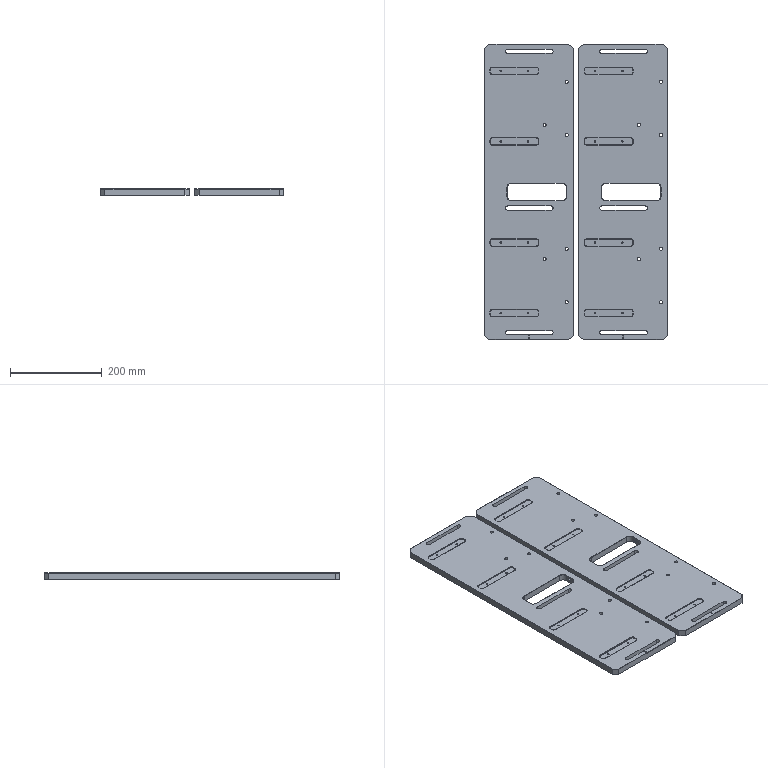NC program | NX | posted by the shop | part box 401 x 645 x 14 mm
Whole program:
%
O0001
(Machine time: 193.92 MIN)
(===Total Tool:5===)
(T2=D6 chamfer mill   D=6.   R=0.   D-  H02 Z=-2.15 )
(T13=ZT3.3  D=3.3  DR_a=118 D-  H13 Z=-18.  )
(T16=ZT6.8  D=6.8  DR_a=118 D-  H16 Z=-23.04)
(T21=M4X0.7 D=3.3  DR_a=180 D-  H21 Z=-0.   )
(T19=M8X1.25 D=6.8  DR_a=180 D-  H19 Z=-18.  )
G80 G90 G17 G49 G40
G91 G28 Z0
M01
N1 T02 M06
(D6 chamfer mill  D=6. R=0. H=02 ce=0.00 di=0.00)
G00 G90 G54 X58. Y-159. M03 S8000
G43 H02 Z20.
M08
G98 G81 X58. Y-159. Z-.8 R1. F500.
Y-99.
X82. Y-14.6
X198.
X176. Y-63.1
X212. Y-99.
Y-159.
X433.
Y-99.
X469. Y-63.1
X447. Y-14.6
X563.
X587. Y-99.
Y-159.
G80
G00 Z20.
G91 G28 Z0.0
M05
M09
G91 G28 Z0.0
M01
N2 T13 M06
(ZT3.3 D=3.3 DR_a=118 H=13)
G00 G90 G54 X58. Y-159. M03 S3000
G43 H13 Z20.
M08
G98 G83 X58. Y-159. Z-18. R1. F300. Q2.
Y-99.
X212.
Y-159.
X433.
Y-99.
X587.
Y-159.
G80
G00 Z20.
G91 G28 Z0.0
M05
M09
G91 G28 Z0.0
M01
N3 T16 M06
(ZT6.8 D=6.8 DR_a=118 H=16)
G00 G90 G54 X563. Y-14.6 M03 S1800
G43 H16 Z20.
M08
G98 G83 X563. Y-14.6 Z-23.043 R1. F350. Q3.
X469. Y-63.1
X447. Y-14.6
X198.
X176. Y-63.1
X82. Y-14.6
G80
G00 Z20.
G91 G28 Z0.0
M05
M09
G91 G28 Z0.0
M01
N4 T02 M06
(D6 chamfer mill  D=6. R=0. H=02 ce=0.00 di=0.00)
G00 G90 G54 X58. Y-159. M03 S8000
G43 H02 Z20.
M08
G98 G81 X58. Y-159. Z-2.15 R3. F500.
Y-99.
X212.
Y-159.
X433.
Y-99.
X587.
Y-159.
G80
G00 Z20.
G00 G90 X564.5 Y-13.434 M03 S8000
Z20.
Z-.8
G01 Z-1.3 F600.
Y-13.2
G03 X563. Y-11.7 I-1.5 J0.0
X560.1 Y-14.6 I0.0 J-2.9
X563. Y-17.5 I2.9 J0.0
X565.9 Y-14.6 I0.0 J2.9
X563. Y-11.7 I-2.9 J0.0
X561.5 Y-13.2 I0.0 J-1.5
G01 Y-13.434
Z-.8
G00 Z20.
X470.5 Y-61.934
Z-.8
G01 Z-1.3
Y-61.7
G03 X469. Y-60.2 I-1.5 J0.0
X466.1 Y-63.1 I0.0 J-2.9
X469. Y-66. I2.9 J0.0
X471.9 Y-63.1 I0.0 J2.9
X469. Y-60.2 I-2.9 J0.0
X467.5 Y-61.7 I0.0 J-1.5
G01 Y-61.934
Z-.8
G00 Z20.
X448.5 Y-13.434
Z-.8
G01 Z-1.3
Y-13.2
G03 X447. Y-11.7 I-1.5 J0.0
X444.1 Y-14.6 I0.0 J-2.9
X447. Y-17.5 I2.9 J0.0
X449.9 Y-14.6 I0.0 J2.9
X447. Y-11.7 I-2.9 J0.0
X445.5 Y-13.2 I0.0 J-1.5
G01 Y-13.434
Z-.8
G00 Z20.
X199.5
Z-.8
G01 Z-1.3
Y-13.2
G03 X198. Y-11.7 I-1.5 J0.0
X195.1 Y-14.6 I0.0 J-2.9
X198. Y-17.5 I2.9 J0.0
X200.9 Y-14.6 I0.0 J2.9
X198. Y-11.7 I-2.9 J0.0
X196.5 Y-13.2 I0.0 J-1.5
G01 Y-13.434
Z-.8
G00 Z20.
X177.5 Y-61.934
Z-.8
G01 Z-1.3
Y-61.7
G03 X176. Y-60.2 I-1.5 J0.0
X173.1 Y-63.1 I0.0 J-2.9
X176. Y-66. I2.9 J0.0
X178.9 Y-63.1 I0.0 J2.9
X176. Y-60.2 I-2.9 J0.0
X174.5 Y-61.7 I0.0 J-1.5
G01 Y-61.934
Z-.8
G00 Z20.
X83.5 Y-13.434
Z-.8
G01 Z-1.3
Y-13.2
G03 X82. Y-11.7 I-1.5 J0.0
X79.1 Y-14.6 I0.0 J-2.9
X82. Y-17.5 I2.9 J0.0
X84.9 Y-14.6 I0.0 J2.9
X82. Y-11.7 I-2.9 J0.0
X80.5 Y-13.2 I0.0 J-1.5
G01 Y-13.434
Z-.8
G00 Z20.
G00 G90 X11.584 Y-145.127 M03 S7000
Z20.
Z2.5
G01 X11.66 Y-145.351 Z2.414 F1500.
X11.836 Y-145.724 Z2.264
X12.054 Y-146.075 Z2.113
X12.311 Y-146.398 Z1.963
X12.602 Y-146.689 Z1.813
X12.925 Y-146.946 Z1.663
X13.276 Y-147.164 Z1.513
X13.649 Y-147.34 Z1.363
X14.039 Y-147.473 Z1.213
X14.442 Y-147.56 Z1.062
X14.853 Y-147.6 Z.912
X15.147 Z.805
X15.558 Y-147.56 Z.655
X15.961 Y-147.473 Z.505
X16.351 Y-147.34 Z.355
X16.724 Y-147.164 Z.205
X17.075 Y-146.946 Z.055
X17.398 Y-146.689 Z-.096
X17.689 Y-146.398 Z-.246
X17.946 Y-146.075 Z-.396
X18.164 Y-145.724 Z-.546
X18.34 Y-145.351 Z-.696
X18.473 Y-144.961 Z-.846
X18.56 Y-144.558 Z-.996
X18.6 Y-144.147 Z-1.146
Y-144. Z-1.2
Y-49.
G03 X15. Y-45.4 I-3.6 J0.0
X11.4 Y-49. I0.0 J-3.6
G01 Y-144.
G03 X15. Y-147.6 I3.6 J0.0
X18.6 Y-144. I0.0 J3.6
G01 Y-143.5
Z1.3
G00 Z20.
X284.084 Y-145.127
Z2.5
G01 X284.16 Y-145.351 Z2.414
X284.336 Y-145.724 Z2.264
X284.554 Y-146.075 Z2.113
X284.811 Y-146.398 Z1.963
X285.102 Y-146.689 Z1.813
X285.425 Y-146.946 Z1.663
X285.776 Y-147.164 Z1.513
X286.149 Y-147.34 Z1.363
X286.539 Y-147.473 Z1.213
X286.942 Y-147.56 Z1.062
X287.353 Y-147.6 Z.912
X287.647 Z.805
X288.058 Y-147.56 Z.655
X288.461 Y-147.473 Z.505
X288.851 Y-147.34 Z.355
X289.224 Y-147.164 Z.205
X289.575 Y-146.946 Z.055
X289.898 Y-146.689 Z-.096
X290.189 Y-146.398 Z-.246
X290.446 Y-146.075 Z-.396
X290.664 Y-145.724 Z-.546
X290.84 Y-145.351 Z-.696
X290.973 Y-144.961 Z-.846
X291.06 Y-144.558 Z-.996
X291.1 Y-144.147 Z-1.146
Y-144. Z-1.2
Y-49.
G03 X287.5 Y-45.4 I-3.6 J0.0
X283.9 Y-49. I0.0 J-3.6
G01 Y-144.
G03 X287.5 Y-147.6 I3.6 J0.0
X291.1 Y-144. I0.0 J3.6
G01 Y-143.5
Z1.3
G00 Z20.
X625.654 Y.9
Z2.5
G01 X634.876 Z-.856
X634.961 Z-.887
X635.152 Y.871 Z-.958
X635.336 Y.811 Z-1.028
X635.508 Y.723 Z-1.099
X635.664 Y.609 Z-1.169
X635.724 Y.549 Z-1.2
X645.549 Y-9.276
G02 X645.9 Y-10.124 I-.849 J-.849
G01 Y-184.876
G02 X645.549 Y-185.724 I-1.2 J0.0
G01 X635.724 Y-195.549
G02 X634.876 Y-195.9 I-.849 J.849
G01 X10.124
G02 X9.276 Y-195.549 I0.0 J1.2
G01 X-.549 Y-185.724
G02 X-.9 Y-184.876 I.849 J.849
G01 Y-10.124
G02 X-.549 Y-9.276 I1.2 J0.0
G01 X9.276 Y.549
G02 X10.124 Y.9 I.849 J-.849
G01 X634.876
G02 X635.724 Y.549 I0.0 J-1.2
G01 X636.078 Y.195
Z1.3
G00 Z20.
X321.334 Y-144.1
Z2.5
G01 X331.5 Z-1.2
G03 X340.6 Y-135. I0.0 J9.1
G01 Y-25.
G03 X331.5 Y-15.9 I-9.1 J0.0
G01 X313.5
G03 X304.4 Y-25. I0.0 J-9.1
G01 Y-135.
G03 X313.5 Y-144.1 I9.1 J0.0
G01 X331.5
G03 X332. Y-144.086 I0.0 J9.1
G01 Z1.3
G00 Z20.
X626.4 Y-133.834
Z2.5
G01 Y-144. Z-1.2
G03 X630. Y-147.6 I3.6 J0.0
X633.6 Y-144. I0.0 J3.6
G01 Y-49.
G03 X630. Y-45.4 I-3.6 J0.0
X626.4 Y-49. I0.0 J-3.6
G01 Y-144.
G03 X626.435 Y-144.498 I3.6 J0.0
G01 Z1.3
G00 Z20.
G91 G28 Z0.0
M05
M09
G91 G28 Z0.0
M01
N5 T21 M06
(M4X0.7 D=3.3 DR_a=180 H=21)
G00 G90 G54 X58. Y-159. M03 S600
G43 H21 Z20.
M08
G95
G98 G84 X58. Y-159. Z0.0 R1. F.7 Q4.
Y-99.
X212.
Y-159.
X433.
Y-99.
X587.
Y-159.
G80
G94
G00 Z20.
G91 G28 Z0.0
M05
M09
G91 G28 Z0.0
M01
N6 T19 M06
(M8X1.25 D=6.8 DR_a=180 H=19)
G00 G90 G54 X563. Y-14.6 M03 S500
G43 H19 Z20.
M08
G95
G98 G84 X563. Y-14.6 Z-18. R1. F1.25 Q4.
X469. Y-63.1
X447. Y-14.6
X198.
X176. Y-63.1
X82. Y-14.6
G80
G94
G00 Z20.
M05
M09
G91 G28 Z0.0
G91 G28 Y0.0
M30
%